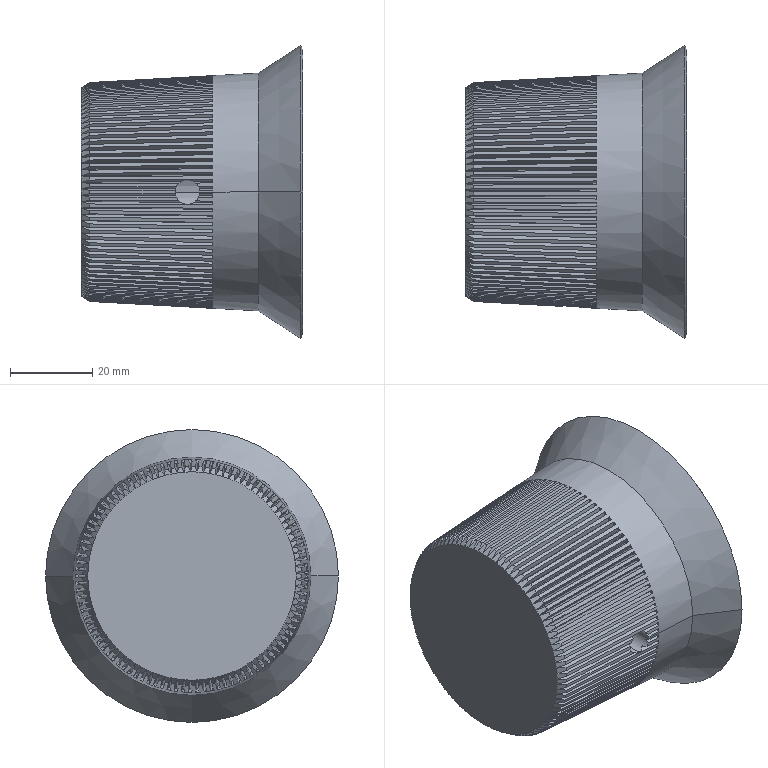Part | SolidWorks | features Chamfer 1, CirPattern 1, ICE 1, Revolution 1, SweepCut 1 | 1 solid | 428 faces | box 53.8 x 71.2 x 71.2 mm | volume 101248 mm3 | plane 312 | cone 112 | cylinder 4 | commonest cylinder face diameters 6 x2 12 x2